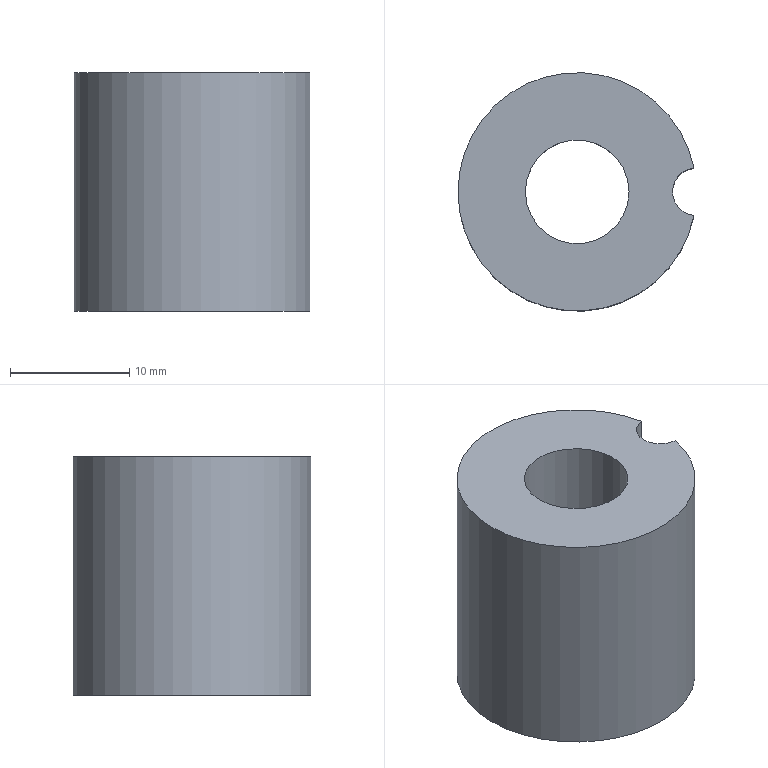Part | NX | features solid 2 | 1 solid | 7 faces | box 19.8 x 20 x 20 mm | volume 4191 mm3 | cylinder 4 | plane 3 | commonest cylinder face diameters 4 x1 8.7 x1 12.6 x1 20 x1
STEP:
#1=CARTESIAN_POINT('',(-310.2,-377.622,-7.));
#2=VERTEX_POINT('',#1);
#3=CARTESIAN_POINT('',(-310.2,-377.622,13.));
#4=VERTEX_POINT('',#3);
#5=CARTESIAN_POINT('',(-310.2,-377.622,3.));
#6=DIRECTION('',(0.,0.,1.));
#7=VECTOR('',#6,1000.);
#8=LINE('',#5,#7);
#9=EDGE_CURVE('',#2,#4,#8,.T.);
#10=ORIENTED_EDGE('',*,*,#9,.F.);
#11=CARTESIAN_POINT('',(-310.2,-381.601,-7.));
#12=VERTEX_POINT('',#11);
#13=CARTESIAN_POINT('',(-320.,-379.611,-7.));
#14=DIRECTION('',(0.,0.,1.));
#15=DIRECTION('',(1.,0.,0.));
#16=AXIS2_PLACEMENT_3D('',#13,#14,#15);
#17=CIRCLE('',#16,10.);
#18=EDGE_CURVE('',#2,#12,#17,.T.);
#19=ORIENTED_EDGE('',*,*,#18,.T.);
#20=CARTESIAN_POINT('',(-310.2,-381.601,13.));
#21=VERTEX_POINT('',#20);
#22=CARTESIAN_POINT('',(-310.2,-381.601,3.));
#23=DIRECTION('',(0.,0.,1.));
#24=VECTOR('',#23,1000.);
#25=LINE('',#22,#24);
#26=EDGE_CURVE('',#21,#12,#25,.F.);
#27=ORIENTED_EDGE('',*,*,#26,.F.);
#28=CARTESIAN_POINT('',(-320.,-379.611,13.));
#29=DIRECTION('',(0.,0.,1.));
#30=DIRECTION('',(1.,0.,0.));
#31=AXIS2_PLACEMENT_3D('',#28,#29,#30);
#32=CIRCLE('',#31,10.);
#33=EDGE_CURVE('',#4,#21,#32,.T.);
#34=ORIENTED_EDGE('',*,*,#33,.F.);
#35=EDGE_LOOP('',(#10,#19,#27,#34));
#36=FACE_BOUND('',#35,.T.);
#37=CARTESIAN_POINT('',(-320.,-379.611,-7.));
#38=DIRECTION('',(0.,0.,1.));
#39=DIRECTION('',(1.,0.,0.));
#40=AXIS2_PLACEMENT_3D('',#37,#38,#39);
#41=CYLINDRICAL_SURFACE('',#40,10.);
#42=ADVANCED_FACE('',(#36),#41,.T.);
#43=CARTESIAN_POINT('',(-313.7,-379.611,-7.));
#44=VERTEX_POINT('',#43);
#45=CARTESIAN_POINT('',(-320.,-379.611,-7.));
#46=DIRECTION('',(0.,0.,1.));
#47=DIRECTION('',(1.,0.,0.));
#48=AXIS2_PLACEMENT_3D('',#45,#46,#47);
#49=CIRCLE('',#48,6.3);
#50=EDGE_CURVE('',#44,#44,#49,.T.);
#51=ORIENTED_EDGE('',*,*,#50,.T.);
#52=EDGE_LOOP('',(#51));
#53=FACE_BOUND('',#52,.T.);
#54=ORIENTED_EDGE('',*,*,#18,.F.);
#55=CARTESIAN_POINT('',(-310.,-379.611,-7.));
#56=DIRECTION('',(0.,0.,1.));
#57=DIRECTION('',(1.,0.,0.));
#58=AXIS2_PLACEMENT_3D('',#55,#56,#57);
#59=CIRCLE('',#58,2.);
#60=EDGE_CURVE('',#2,#12,#59,.T.);
#61=ORIENTED_EDGE('',*,*,#60,.T.);
#62=EDGE_LOOP('',(#54,#61));
#63=FACE_BOUND('',#62,.T.);
#64=CARTESIAN_POINT('',(-320.,-379.611,-7.));
#65=DIRECTION('',(0.,0.,1.));
#66=DIRECTION('',(1.,0.,0.));
#67=AXIS2_PLACEMENT_3D('',#64,#65,#66);
#68=PLANE('',#67);
#69=ADVANCED_FACE('',(#53,#63),#68,.F.);
#70=CARTESIAN_POINT('',(-315.65,-379.611,13.));
#71=VERTEX_POINT('',#70);
#72=CARTESIAN_POINT('',(-320.,-379.611,13.));
#73=DIRECTION('',(0.,0.,1.));
#74=DIRECTION('',(1.,0.,0.));
#75=AXIS2_PLACEMENT_3D('',#72,#73,#74);
#76=CIRCLE('',#75,4.35);
#77=EDGE_CURVE('',#71,#71,#76,.T.);
#78=ORIENTED_EDGE('',*,*,#77,.F.);
#79=EDGE_LOOP('',(#78));
#80=FACE_BOUND('',#79,.T.);
#81=CARTESIAN_POINT('',(-310.,-379.611,13.));
#82=DIRECTION('',(0.,0.,1.));
#83=DIRECTION('',(1.,0.,0.));
#84=AXIS2_PLACEMENT_3D('',#81,#82,#83);
#85=CIRCLE('',#84,2.);
#86=EDGE_CURVE('',#4,#21,#85,.T.);
#87=ORIENTED_EDGE('',*,*,#86,.F.);
#88=ORIENTED_EDGE('',*,*,#33,.T.);
#89=EDGE_LOOP('',(#87,#88));
#90=FACE_BOUND('',#89,.T.);
#91=CARTESIAN_POINT('',(-320.,-379.611,13.));
#92=DIRECTION('',(0.,0.,1.));
#93=DIRECTION('',(1.,0.,0.));
#94=AXIS2_PLACEMENT_3D('',#91,#92,#93);
#95=PLANE('',#94);
#96=ADVANCED_FACE('',(#80,#90),#95,.T.);
#97=ORIENTED_EDGE('',*,*,#50,.F.);
#98=EDGE_LOOP('',(#97));
#99=FACE_BOUND('',#98,.T.);
#100=CARTESIAN_POINT('',(-313.7,-379.611,5.));
#101=VERTEX_POINT('',#100);
#102=CARTESIAN_POINT('',(-320.,-379.611,5.));
#103=DIRECTION('',(0.,0.,1.));
#104=DIRECTION('',(1.,0.,0.));
#105=AXIS2_PLACEMENT_3D('',#102,#103,#104);
#106=CIRCLE('',#105,6.3);
#107=EDGE_CURVE('',#101,#101,#106,.T.);
#108=ORIENTED_EDGE('',*,*,#107,.T.);
#109=EDGE_LOOP('',(#108));
#110=FACE_BOUND('',#109,.T.);
#111=CARTESIAN_POINT('',(-320.,-379.611,-7.));
#112=DIRECTION('',(0.,0.,1.));
#113=DIRECTION('',(1.,0.,0.));
#114=AXIS2_PLACEMENT_3D('',#111,#112,#113);
#115=CYLINDRICAL_SURFACE('',#114,6.3);
#116=ADVANCED_FACE('',(#99,#110),#115,.F.);
#117=CARTESIAN_POINT('',(-315.65,-379.611,5.));
#118=VERTEX_POINT('',#117);
#119=CARTESIAN_POINT('',(-320.,-379.611,5.));
#120=DIRECTION('',(0.,0.,1.));
#121=DIRECTION('',(1.,0.,0.));
#122=AXIS2_PLACEMENT_3D('',#119,#120,#121);
#123=CIRCLE('',#122,4.35);
#124=EDGE_CURVE('',#118,#118,#123,.T.);
#125=ORIENTED_EDGE('',*,*,#124,.T.);
#126=EDGE_LOOP('',(#125));
#127=FACE_BOUND('',#126,.T.);
#128=ORIENTED_EDGE('',*,*,#107,.F.);
#129=EDGE_LOOP('',(#128));
#130=FACE_BOUND('',#129,.T.);
#131=CARTESIAN_POINT('',(-320.,-379.611,5.));
#132=DIRECTION('',(0.,0.,1.));
#133=DIRECTION('',(1.,0.,0.));
#134=AXIS2_PLACEMENT_3D('',#131,#132,#133);
#135=PLANE('',#134);
#136=ADVANCED_FACE('',(#127,#130),#135,.F.);
#137=ORIENTED_EDGE('',*,*,#9,.T.);
#138=ORIENTED_EDGE('',*,*,#86,.T.);
#139=ORIENTED_EDGE('',*,*,#26,.T.);
#140=ORIENTED_EDGE('',*,*,#60,.F.);
#141=EDGE_LOOP('',(#137,#138,#139,#140));
#142=FACE_BOUND('',#141,.T.);
#143=CARTESIAN_POINT('',(-310.,-379.611,-7.));
#144=DIRECTION('',(0.,0.,1.));
#145=DIRECTION('',(1.,0.,0.));
#146=AXIS2_PLACEMENT_3D('',#143,#144,#145);
#147=CYLINDRICAL_SURFACE('',#146,2.);
#148=ADVANCED_FACE('',(#142),#147,.F.);
#149=ORIENTED_EDGE('',*,*,#77,.T.);
#150=EDGE_LOOP('',(#149));
#151=FACE_BOUND('',#150,.T.);
#152=ORIENTED_EDGE('',*,*,#124,.F.);
#153=EDGE_LOOP('',(#152));
#154=FACE_BOUND('',#153,.T.);
#155=CARTESIAN_POINT('',(-320.,-379.611,-7.));
#156=DIRECTION('',(0.,0.,1.));
#157=DIRECTION('',(1.,0.,0.));
#158=AXIS2_PLACEMENT_3D('',#155,#156,#157);
#159=CYLINDRICAL_SURFACE('',#158,4.35);
#160=ADVANCED_FACE('',(#151,#154),#159,.F.);
#161=CLOSED_SHELL('',(#42,#69,#96,#116,#136,#148,#160));
#162=MANIFOLD_SOLID_BREP('',#161);
#163=(LENGTH_UNIT()NAMED_UNIT(*)SI_UNIT(.MILLI.,.METRE.));
#164=UNCERTAINTY_MEASURE_WITH_UNIT(LENGTH_MEASURE(0.00001),#163,'','');
#165=(NAMED_UNIT(*)PLANE_ANGLE_UNIT()SI_UNIT($,.RADIAN.));
#166=(NAMED_UNIT(*)SI_UNIT($,.STERADIAN.)SOLID_ANGLE_UNIT());
#167=(GEOMETRIC_REPRESENTATION_CONTEXT(3)GLOBAL_UNCERTAINTY_ASSIGNED_CONTEXT((#164))GLOBAL_UNIT_ASSIGNED_CONTEXT((#163,#165,#166))REPRESENTATION_CONTEXT('',''));
#168=ADVANCED_BREP_SHAPE_REPRESENTATION('',(#162),#167);